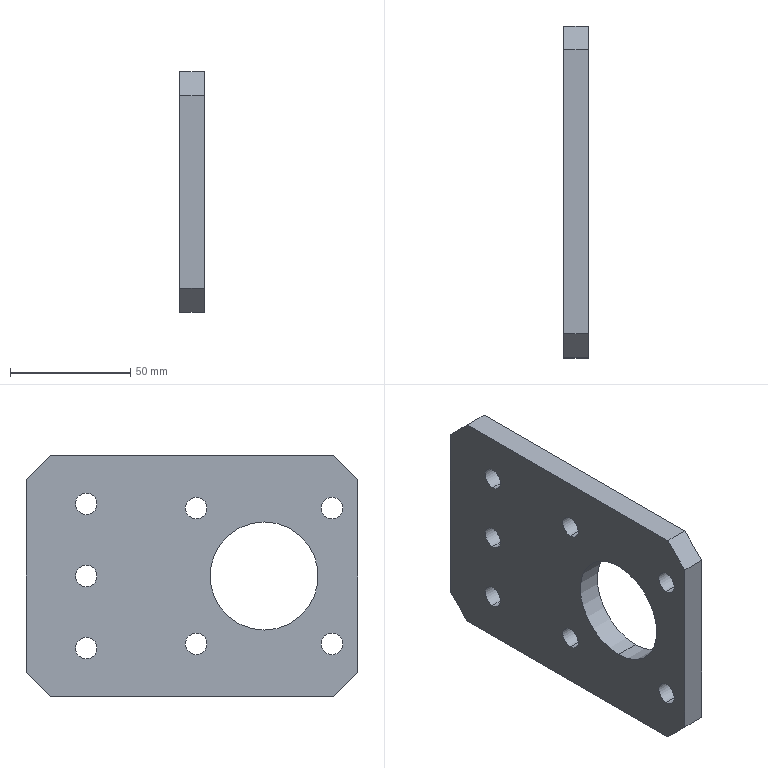Part | SolidWorks | features HoleWzd 2, Chamfer 1, CirPattern 1, Extrusion 1, ICE 1 | 1 solid | 26 faces | box 10 x 138 x 100 mm | volume 115642 mm3 | cylinder 16 | plane 10 | commonest cylinder face diameters 9 x14 45 x2
STEP:
#1=CARTESIAN_POINT('',(0.,-1.75,-23.75));
#2=VERTEX_POINT('',#1);
#3=CARTESIAN_POINT('',(0.,-1.75,-32.75));
#4=VERTEX_POINT('',#3);
#5=CARTESIAN_POINT('',(0.,-1.75,-28.25));
#6=DIRECTION('',(1.,0.,0.));
#7=DIRECTION('',(0.,0.,-1.));
#8=AXIS2_PLACEMENT_3D('',#5,#6,#7);
#9=CIRCLE('',#8,4.5);
#10=EDGE_CURVE('',#2,#4,#9,.T.);
#11=ORIENTED_EDGE('',*,*,#10,.F.);
#12=CARTESIAN_POINT('',(10.,-1.75,-23.75));
#13=VERTEX_POINT('',#12);
#14=CARTESIAN_POINT('',(10.,-1.75,-23.75));
#15=DIRECTION('',(1.,0.,0.));
#16=VECTOR('',#15,1000.);
#17=LINE('',#14,#16);
#18=EDGE_CURVE('',#2,#13,#17,.T.);
#19=ORIENTED_EDGE('',*,*,#18,.T.);
#20=CARTESIAN_POINT('',(10.,-1.75,-32.75));
#21=VERTEX_POINT('',#20);
#22=CARTESIAN_POINT('',(10.,-1.75,-28.25));
#23=DIRECTION('',(1.,0.,0.));
#24=DIRECTION('',(0.,0.,-1.));
#25=AXIS2_PLACEMENT_3D('',#22,#23,#24);
#26=CIRCLE('',#25,4.5);
#27=EDGE_CURVE('',#13,#21,#26,.T.);
#28=ORIENTED_EDGE('',*,*,#27,.T.);
#29=CARTESIAN_POINT('',(10.,-1.75,-32.75));
#30=DIRECTION('',(1.,0.,0.));
#31=VECTOR('',#30,1000.);
#32=LINE('',#29,#31);
#33=EDGE_CURVE('',#4,#21,#32,.T.);
#34=ORIENTED_EDGE('',*,*,#33,.F.);
#35=EDGE_LOOP('',(#11,#19,#28,#34));
#36=FACE_OUTER_BOUND('',#35,.T.);
#37=CARTESIAN_POINT('',(10.,-1.75,-28.25));
#38=DIRECTION('',(1.,0.,0.));
#39=DIRECTION('',(0.,0.,-1.));
#40=AXIS2_PLACEMENT_3D('',#37,#38,#39);
#41=CYLINDRICAL_SURFACE('',#40,4.5);
#42=ADVANCED_FACE('',(#36),#41,.F.);
#43=CARTESIAN_POINT('',(0.,-58.25,-23.75));
#44=VERTEX_POINT('',#43);
#45=CARTESIAN_POINT('',(0.,-58.25,-32.75));
#46=VERTEX_POINT('',#45);
#47=CARTESIAN_POINT('',(0.,-58.25,-28.25));
#48=DIRECTION('',(1.,0.,0.));
#49=DIRECTION('',(0.,0.,-1.));
#50=AXIS2_PLACEMENT_3D('',#47,#48,#49);
#51=CIRCLE('',#50,4.5);
#52=EDGE_CURVE('',#44,#46,#51,.T.);
#53=ORIENTED_EDGE('',*,*,#52,.F.);
#54=CARTESIAN_POINT('',(10.,-58.25,-23.75));
#55=VERTEX_POINT('',#54);
#56=CARTESIAN_POINT('',(10.,-58.25,-23.75));
#57=DIRECTION('',(1.,0.,0.));
#58=VECTOR('',#57,1000.);
#59=LINE('',#56,#58);
#60=EDGE_CURVE('',#44,#55,#59,.T.);
#61=ORIENTED_EDGE('',*,*,#60,.T.);
#62=CARTESIAN_POINT('',(10.,-58.25,-32.75));
#63=VERTEX_POINT('',#62);
#64=CARTESIAN_POINT('',(10.,-58.25,-28.25));
#65=DIRECTION('',(1.,0.,0.));
#66=DIRECTION('',(0.,0.,-1.));
#67=AXIS2_PLACEMENT_3D('',#64,#65,#66);
#68=CIRCLE('',#67,4.5);
#69=EDGE_CURVE('',#55,#63,#68,.T.);
#70=ORIENTED_EDGE('',*,*,#69,.T.);
#71=CARTESIAN_POINT('',(10.,-58.25,-32.75));
#72=DIRECTION('',(1.,0.,0.));
#73=VECTOR('',#72,1000.);
#74=LINE('',#71,#73);
#75=EDGE_CURVE('',#46,#63,#74,.T.);
#76=ORIENTED_EDGE('',*,*,#75,.F.);
#77=EDGE_LOOP('',(#53,#61,#70,#76));
#78=FACE_OUTER_BOUND('',#77,.T.);
#79=CARTESIAN_POINT('',(10.,-58.25,-28.25));
#80=DIRECTION('',(1.,0.,0.));
#81=DIRECTION('',(0.,0.,-1.));
#82=AXIS2_PLACEMENT_3D('',#79,#80,#81);
#83=CYLINDRICAL_SURFACE('',#82,4.5);
#84=ADVANCED_FACE('',(#78),#83,.F.);
#85=CARTESIAN_POINT('',(0.,-58.25,32.75));
#86=VERTEX_POINT('',#85);
#87=CARTESIAN_POINT('',(0.,-58.25,23.75));
#88=VERTEX_POINT('',#87);
#89=CARTESIAN_POINT('',(0.,-58.25,28.25));
#90=DIRECTION('',(1.,0.,0.));
#91=DIRECTION('',(0.,0.,-1.));
#92=AXIS2_PLACEMENT_3D('',#89,#90,#91);
#93=CIRCLE('',#92,4.5);
#94=EDGE_CURVE('',#86,#88,#93,.T.);
#95=ORIENTED_EDGE('',*,*,#94,.F.);
#96=CARTESIAN_POINT('',(10.,-58.25,32.75));
#97=VERTEX_POINT('',#96);
#98=CARTESIAN_POINT('',(10.,-58.25,32.75));
#99=DIRECTION('',(1.,0.,0.));
#100=VECTOR('',#99,1000.);
#101=LINE('',#98,#100);
#102=EDGE_CURVE('',#86,#97,#101,.T.);
#103=ORIENTED_EDGE('',*,*,#102,.T.);
#104=CARTESIAN_POINT('',(10.,-58.25,23.75));
#105=VERTEX_POINT('',#104);
#106=CARTESIAN_POINT('',(10.,-58.25,28.25));
#107=DIRECTION('',(1.,0.,0.));
#108=DIRECTION('',(0.,0.,-1.));
#109=AXIS2_PLACEMENT_3D('',#106,#107,#108);
#110=CIRCLE('',#109,4.5);
#111=EDGE_CURVE('',#97,#105,#110,.T.);
#112=ORIENTED_EDGE('',*,*,#111,.T.);
#113=CARTESIAN_POINT('',(10.,-58.25,23.75));
#114=DIRECTION('',(1.,0.,0.));
#115=VECTOR('',#114,1000.);
#116=LINE('',#113,#115);
#117=EDGE_CURVE('',#88,#105,#116,.T.);
#118=ORIENTED_EDGE('',*,*,#117,.F.);
#119=EDGE_LOOP('',(#95,#103,#112,#118));
#120=FACE_OUTER_BOUND('',#119,.T.);
#121=CARTESIAN_POINT('',(10.,-58.25,28.25));
#122=DIRECTION('',(1.,0.,0.));
#123=DIRECTION('',(0.,0.,-1.));
#124=AXIS2_PLACEMENT_3D('',#121,#122,#123);
#125=CYLINDRICAL_SURFACE('',#124,4.5);
#126=ADVANCED_FACE('',(#120),#125,.F.);
#127=CARTESIAN_POINT('',(0.,-1.75,32.75));
#128=VERTEX_POINT('',#127);
#129=CARTESIAN_POINT('',(0.,-1.75,23.75));
#130=VERTEX_POINT('',#129);
#131=CARTESIAN_POINT('',(0.,-1.75,28.25));
#132=DIRECTION('',(1.,0.,0.));
#133=DIRECTION('',(0.,0.,-1.));
#134=AXIS2_PLACEMENT_3D('',#131,#132,#133);
#135=CIRCLE('',#134,4.5);
#136=EDGE_CURVE('',#128,#130,#135,.T.);
#137=ORIENTED_EDGE('',*,*,#136,.F.);
#138=CARTESIAN_POINT('',(10.,-1.75,32.75));
#139=VERTEX_POINT('',#138);
#140=CARTESIAN_POINT('',(10.,-1.75,32.75));
#141=DIRECTION('',(1.,0.,0.));
#142=VECTOR('',#141,1000.);
#143=LINE('',#140,#142);
#144=EDGE_CURVE('',#128,#139,#143,.T.);
#145=ORIENTED_EDGE('',*,*,#144,.T.);
#146=CARTESIAN_POINT('',(10.,-1.75,23.75));
#147=VERTEX_POINT('',#146);
#148=CARTESIAN_POINT('',(10.,-1.75,28.25));
#149=DIRECTION('',(1.,0.,0.));
#150=DIRECTION('',(0.,0.,-1.));
#151=AXIS2_PLACEMENT_3D('',#148,#149,#150);
#152=CIRCLE('',#151,4.5);
#153=EDGE_CURVE('',#139,#147,#152,.T.);
#154=ORIENTED_EDGE('',*,*,#153,.T.);
#155=CARTESIAN_POINT('',(10.,-1.75,23.75));
#156=DIRECTION('',(1.,0.,0.));
#157=VECTOR('',#156,1000.);
#158=LINE('',#155,#157);
#159=EDGE_CURVE('',#130,#147,#158,.T.);
#160=ORIENTED_EDGE('',*,*,#159,.F.);
#161=EDGE_LOOP('',(#137,#145,#154,#160));
#162=FACE_OUTER_BOUND('',#161,.T.);
#163=CARTESIAN_POINT('',(10.,-1.75,28.25));
#164=DIRECTION('',(1.,0.,0.));
#165=DIRECTION('',(0.,0.,-1.));
#166=AXIS2_PLACEMENT_3D('',#163,#164,#165);
#167=CYLINDRICAL_SURFACE('',#166,4.5);
#168=ADVANCED_FACE('',(#162),#167,.F.);
#169=CARTESIAN_POINT('',(0.,-30.,22.5));
#170=VERTEX_POINT('',#169);
#171=CARTESIAN_POINT('',(0.,-30.,-22.5));
#172=VERTEX_POINT('',#171);
#173=CARTESIAN_POINT('',(0.,-30.,0.));
#174=DIRECTION('',(1.,0.,0.));
#175=DIRECTION('',(0.,0.,-1.));
#176=AXIS2_PLACEMENT_3D('',#173,#174,#175);
#177=CIRCLE('',#176,22.5);
#178=EDGE_CURVE('',#170,#172,#177,.T.);
#179=ORIENTED_EDGE('',*,*,#178,.F.);
#180=CARTESIAN_POINT('',(10.,-30.,22.5));
#181=VERTEX_POINT('',#180);
#182=CARTESIAN_POINT('',(0.,-30.,22.5));
#183=DIRECTION('',(1.,0.,0.));
#184=VECTOR('',#183,1000.);
#185=LINE('',#182,#184);
#186=EDGE_CURVE('',#170,#181,#185,.T.);
#187=ORIENTED_EDGE('',*,*,#186,.T.);
#188=CARTESIAN_POINT('',(10.,-30.,-22.5));
#189=VERTEX_POINT('',#188);
#190=CARTESIAN_POINT('',(10.,-30.,0.));
#191=DIRECTION('',(1.,0.,0.));
#192=DIRECTION('',(0.,0.,-1.));
#193=AXIS2_PLACEMENT_3D('',#190,#191,#192);
#194=CIRCLE('',#193,22.5);
#195=EDGE_CURVE('',#181,#189,#194,.T.);
#196=ORIENTED_EDGE('',*,*,#195,.T.);
#197=CARTESIAN_POINT('',(0.,-30.,-22.5));
#198=DIRECTION('',(1.,0.,0.));
#199=VECTOR('',#198,1000.);
#200=LINE('',#197,#199);
#201=EDGE_CURVE('',#172,#189,#200,.T.);
#202=ORIENTED_EDGE('',*,*,#201,.F.);
#203=EDGE_LOOP('',(#179,#187,#196,#202));
#204=FACE_OUTER_BOUND('',#203,.T.);
#205=CARTESIAN_POINT('',(0.,-30.,0.));
#206=DIRECTION('',(1.,0.,0.));
#207=DIRECTION('',(0.,0.,-1.));
#208=AXIS2_PLACEMENT_3D('',#205,#206,#207);
#209=CYLINDRICAL_SURFACE('',#208,22.5);
#210=ADVANCED_FACE('',(#204),#209,.F.);
#211=CARTESIAN_POINT('',(0.,44.,34.5));
#212=VERTEX_POINT('',#211);
#213=CARTESIAN_POINT('',(0.,44.,25.5));
#214=VERTEX_POINT('',#213);
#215=CARTESIAN_POINT('',(0.,44.,30.));
#216=DIRECTION('',(1.,0.,0.));
#217=DIRECTION('',(0.,0.,-1.));
#218=AXIS2_PLACEMENT_3D('',#215,#216,#217);
#219=CIRCLE('',#218,4.5);
#220=EDGE_CURVE('',#212,#214,#219,.T.);
#221=ORIENTED_EDGE('',*,*,#220,.F.);
#222=CARTESIAN_POINT('',(10.,44.,34.5));
#223=VERTEX_POINT('',#222);
#224=CARTESIAN_POINT('',(10.,44.,34.5));
#225=DIRECTION('',(1.,0.,0.));
#226=VECTOR('',#225,1000.);
#227=LINE('',#224,#226);
#228=EDGE_CURVE('',#212,#223,#227,.T.);
#229=ORIENTED_EDGE('',*,*,#228,.T.);
#230=CARTESIAN_POINT('',(10.,44.,25.5));
#231=VERTEX_POINT('',#230);
#232=CARTESIAN_POINT('',(10.,44.,30.));
#233=DIRECTION('',(1.,0.,0.));
#234=DIRECTION('',(0.,0.,-1.));
#235=AXIS2_PLACEMENT_3D('',#232,#233,#234);
#236=CIRCLE('',#235,4.5);
#237=EDGE_CURVE('',#223,#231,#236,.T.);
#238=ORIENTED_EDGE('',*,*,#237,.T.);
#239=CARTESIAN_POINT('',(10.,44.,25.5));
#240=DIRECTION('',(1.,0.,0.));
#241=VECTOR('',#240,1000.);
#242=LINE('',#239,#241);
#243=EDGE_CURVE('',#214,#231,#242,.T.);
#244=ORIENTED_EDGE('',*,*,#243,.F.);
#245=EDGE_LOOP('',(#221,#229,#238,#244));
#246=FACE_OUTER_BOUND('',#245,.T.);
#247=CARTESIAN_POINT('',(10.,44.,30.));
#248=DIRECTION('',(1.,0.,0.));
#249=DIRECTION('',(0.,0.,-1.));
#250=AXIS2_PLACEMENT_3D('',#247,#248,#249);
#251=CYLINDRICAL_SURFACE('',#250,4.5);
#252=ADVANCED_FACE('',(#246),#251,.F.);
#253=CARTESIAN_POINT('',(0.,44.,4.5));
#254=VERTEX_POINT('',#253);
#255=CARTESIAN_POINT('',(0.,44.,-4.5));
#256=VERTEX_POINT('',#255);
#257=CARTESIAN_POINT('',(0.,44.,0.));
#258=DIRECTION('',(1.,0.,0.));
#259=DIRECTION('',(0.,0.,-1.));
#260=AXIS2_PLACEMENT_3D('',#257,#258,#259);
#261=CIRCLE('',#260,4.5);
#262=EDGE_CURVE('',#254,#256,#261,.T.);
#263=ORIENTED_EDGE('',*,*,#262,.F.);
#264=CARTESIAN_POINT('',(10.,44.,4.5));
#265=VERTEX_POINT('',#264);
#266=CARTESIAN_POINT('',(10.,44.,4.5));
#267=DIRECTION('',(1.,0.,0.));
#268=VECTOR('',#267,1000.);
#269=LINE('',#266,#268);
#270=EDGE_CURVE('',#254,#265,#269,.T.);
#271=ORIENTED_EDGE('',*,*,#270,.T.);
#272=CARTESIAN_POINT('',(10.,44.,-4.5));
#273=VERTEX_POINT('',#272);
#274=CARTESIAN_POINT('',(10.,44.,0.));
#275=DIRECTION('',(1.,0.,0.));
#276=DIRECTION('',(0.,0.,-1.));
#277=AXIS2_PLACEMENT_3D('',#274,#275,#276);
#278=CIRCLE('',#277,4.5);
#279=EDGE_CURVE('',#265,#273,#278,.T.);
#280=ORIENTED_EDGE('',*,*,#279,.T.);
#281=CARTESIAN_POINT('',(10.,44.,-4.5));
#282=DIRECTION('',(1.,0.,0.));
#283=VECTOR('',#282,1000.);
#284=LINE('',#281,#283);
#285=EDGE_CURVE('',#256,#273,#284,.T.);
#286=ORIENTED_EDGE('',*,*,#285,.F.);
#287=EDGE_LOOP('',(#263,#271,#280,#286));
#288=FACE_OUTER_BOUND('',#287,.T.);
#289=CARTESIAN_POINT('',(10.,44.,0.));
#290=DIRECTION('',(1.,0.,0.));
#291=DIRECTION('',(0.,0.,-1.));
#292=AXIS2_PLACEMENT_3D('',#289,#290,#291);
#293=CYLINDRICAL_SURFACE('',#292,4.5);
#294=ADVANCED_FACE('',(#288),#293,.F.);
#295=CARTESIAN_POINT('',(0.,44.,-25.5));
#296=VERTEX_POINT('',#295);
#297=CARTESIAN_POINT('',(0.,44.,-34.5));
#298=VERTEX_POINT('',#297);
#299=CARTESIAN_POINT('',(0.,44.,-30.));
#300=DIRECTION('',(1.,0.,0.));
#301=DIRECTION('',(0.,0.,-1.));
#302=AXIS2_PLACEMENT_3D('',#299,#300,#301);
#303=CIRCLE('',#302,4.5);
#304=EDGE_CURVE('',#296,#298,#303,.T.);
#305=ORIENTED_EDGE('',*,*,#304,.F.);
#306=CARTESIAN_POINT('',(10.,44.,-25.5));
#307=VERTEX_POINT('',#306);
#308=CARTESIAN_POINT('',(10.,44.,-25.5));
#309=DIRECTION('',(1.,0.,0.));
#310=VECTOR('',#309,1000.);
#311=LINE('',#308,#310);
#312=EDGE_CURVE('',#296,#307,#311,.T.);
#313=ORIENTED_EDGE('',*,*,#312,.T.);
#314=CARTESIAN_POINT('',(10.,44.,-34.5));
#315=VERTEX_POINT('',#314);
#316=CARTESIAN_POINT('',(10.,44.,-30.));
#317=DIRECTION('',(1.,0.,0.));
#318=DIRECTION('',(0.,0.,-1.));
#319=AXIS2_PLACEMENT_3D('',#316,#317,#318);
#320=CIRCLE('',#319,4.5);
#321=EDGE_CURVE('',#307,#315,#320,.T.);
#322=ORIENTED_EDGE('',*,*,#321,.T.);
#323=CARTESIAN_POINT('',(10.,44.,-34.5));
#324=DIRECTION('',(1.,0.,0.));
#325=VECTOR('',#324,1000.);
#326=LINE('',#323,#325);
#327=EDGE_CURVE('',#298,#315,#326,.T.);
#328=ORIENTED_EDGE('',*,*,#327,.F.);
#329=EDGE_LOOP('',(#305,#313,#322,#328));
#330=FACE_OUTER_BOUND('',#329,.T.);
#331=CARTESIAN_POINT('',(10.,44.,-30.));
#332=DIRECTION('',(1.,0.,0.));
#333=DIRECTION('',(0.,0.,-1.));
#334=AXIS2_PLACEMENT_3D('',#331,#332,#333);
#335=CYLINDRICAL_SURFACE('',#334,4.5);
#336=ADVANCED_FACE('',(#330),#335,.F.);
#337=CARTESIAN_POINT('',(10.,-59.,-50.));
#338=VERTEX_POINT('',#337);
#339=CARTESIAN_POINT('',(10.,59.,-50.));
#340=VERTEX_POINT('',#339);
#341=CARTESIAN_POINT('',(10.,69.,-50.));
#342=DIRECTION('',(0.,1.,0.));
#343=VECTOR('',#342,1000.);
#344=LINE('',#341,#343);
#345=EDGE_CURVE('',#338,#340,#344,.T.);
#346=ORIENTED_EDGE('',*,*,#345,.F.);
#347=CARTESIAN_POINT('',(0.,-59.,-50.));
#348=VERTEX_POINT('',#347);
#349=CARTESIAN_POINT('',(10.,-59.,-50.));
#350=DIRECTION('',(-1.,0.,0.));
#351=VECTOR('',#350,1000.);
#352=LINE('',#349,#351);
#353=EDGE_CURVE('',#338,#348,#352,.T.);
#354=ORIENTED_EDGE('',*,*,#353,.T.);
#355=CARTESIAN_POINT('',(0.,59.,-50.));
#356=VERTEX_POINT('',#355);
#357=CARTESIAN_POINT('',(0.,69.,-50.));
#358=DIRECTION('',(0.,1.,0.));
#359=VECTOR('',#358,1000.);
#360=LINE('',#357,#359);
#361=EDGE_CURVE('',#348,#356,#360,.T.);
#362=ORIENTED_EDGE('',*,*,#361,.T.);
#363=CARTESIAN_POINT('',(10.,59.,-50.));
#364=DIRECTION('',(1.,0.,0.));
#365=VECTOR('',#364,1000.);
#366=LINE('',#363,#365);
#367=EDGE_CURVE('',#356,#340,#366,.T.);
#368=ORIENTED_EDGE('',*,*,#367,.T.);
#369=EDGE_LOOP('',(#346,#354,#362,#368));
#370=FACE_OUTER_BOUND('',#369,.T.);
#371=CARTESIAN_POINT('',(10.,69.,-50.));
#372=DIRECTION('',(0.,0.,1.));
#373=DIRECTION('',(0.,-1.,0.));
#374=AXIS2_PLACEMENT_3D('',#371,#372,#373);
#375=PLANE('',#374);
#376=ADVANCED_FACE('',(#370),#375,.F.);
#377=CARTESIAN_POINT('',(10.,69.,-40.));
#378=VERTEX_POINT('',#377);
#379=CARTESIAN_POINT('',(10.,69.,40.));
#380=VERTEX_POINT('',#379);
#381=CARTESIAN_POINT('',(10.,69.,50.));
#382=DIRECTION('',(0.,0.,1.));
#383=VECTOR('',#382,1000.);
#384=LINE('',#381,#383);
#385=EDGE_CURVE('',#378,#380,#384,.T.);
#386=ORIENTED_EDGE('',*,*,#385,.F.);
#387=CARTESIAN_POINT('',(0.,69.,-40.));
#388=VERTEX_POINT('',#387);
#389=CARTESIAN_POINT('',(10.,69.,-40.));
#390=DIRECTION('',(-1.,0.,0.));
#391=VECTOR('',#390,1000.);
#392=LINE('',#389,#391);
#393=EDGE_CURVE('',#378,#388,#392,.T.);
#394=ORIENTED_EDGE('',*,*,#393,.T.);
#395=CARTESIAN_POINT('',(0.,69.,40.));
#396=VERTEX_POINT('',#395);
#397=CARTESIAN_POINT('',(0.,69.,50.));
#398=DIRECTION('',(0.,0.,1.));
#399=VECTOR('',#398,1000.);
#400=LINE('',#397,#399);
#401=EDGE_CURVE('',#388,#396,#400,.T.);
#402=ORIENTED_EDGE('',*,*,#401,.T.);
#403=CARTESIAN_POINT('',(10.,69.,40.));
#404=DIRECTION('',(1.,0.,0.));
#405=VECTOR('',#404,1000.);
#406=LINE('',#403,#405);
#407=EDGE_CURVE('',#396,#380,#406,.T.);
#408=ORIENTED_EDGE('',*,*,#407,.T.);
#409=EDGE_LOOP('',(#386,#394,#402,#408));
#410=FACE_OUTER_BOUND('',#409,.T.);
#411=CARTESIAN_POINT('',(10.,69.,50.));
#412=DIRECTION('',(0.,-1.,0.));
#413=DIRECTION('',(0.,0.,-1.));
#414=AXIS2_PLACEMENT_3D('',#411,#412,#413);
#415=PLANE('',#414);
#416=ADVANCED_FACE('',(#410),#415,.F.);
#417=CARTESIAN_POINT('',(0.,59.,50.));
#418=VERTEX_POINT('',#417);
#419=CARTESIAN_POINT('',(0.,-59.,50.));
#420=VERTEX_POINT('',#419);
#421=CARTESIAN_POINT('',(0.,69.,50.));
#422=DIRECTION('',(0.,-1.,0.));
#423=VECTOR('',#422,1000.);
#424=LINE('',#421,#423);
#425=EDGE_CURVE('',#418,#420,#424,.T.);
#426=ORIENTED_EDGE('',*,*,#425,.T.);
#427=CARTESIAN_POINT('',(10.,-59.,50.));
#428=VERTEX_POINT('',#427);
#429=CARTESIAN_POINT('',(10.,-59.,50.));
#430=DIRECTION('',(1.,0.,0.));
#431=VECTOR('',#430,1000.);
#432=LINE('',#429,#431);
#433=EDGE_CURVE('',#420,#428,#432,.T.);
#434=ORIENTED_EDGE('',*,*,#433,.T.);
#435=CARTESIAN_POINT('',(10.,59.,50.));
#436=VERTEX_POINT('',#435);
#437=CARTESIAN_POINT('',(10.,69.,50.));
#438=DIRECTION('',(0.,-1.,0.));
#439=VECTOR('',#438,1000.);
#440=LINE('',#437,#439);
#441=EDGE_CURVE('',#436,#428,#440,.T.);
#442=ORIENTED_EDGE('',*,*,#441,.F.);
#443=CARTESIAN_POINT('',(10.,59.,50.));
#444=DIRECTION('',(-1.,0.,0.));
#445=VECTOR('',#444,1000.);
#446=LINE('',#443,#445);
#447=EDGE_CURVE('',#436,#418,#446,.T.);
#448=ORIENTED_EDGE('',*,*,#447,.T.);
#449=EDGE_LOOP('',(#426,#434,#442,#448));
#450=FACE_OUTER_BOUND('',#449,.T.);
#451=CARTESIAN_POINT('',(10.,69.,50.));
#452=DIRECTION('',(0.,0.,-1.));
#453=DIRECTION('',(0.,1.,0.));
#454=AXIS2_PLACEMENT_3D('',#451,#452,#453);
#455=PLANE('',#454);
#456=ADVANCED_FACE('',(#450),#455,.F.);
#457=CARTESIAN_POINT('',(10.,-69.,40.));
#458=VERTEX_POINT('',#457);
#459=CARTESIAN_POINT('',(10.,-69.,-40.));
#460=VERTEX_POINT('',#459);
#461=CARTESIAN_POINT('',(10.,-69.,50.));
#462=DIRECTION('',(0.,0.,-1.));
#463=VECTOR('',#462,1000.);
#464=LINE('',#461,#463);
#465=EDGE_CURVE('',#458,#460,#464,.T.);
#466=ORIENTED_EDGE('',*,*,#465,.F.);
#467=CARTESIAN_POINT('',(0.,-69.,40.));
#468=VERTEX_POINT('',#467);
#469=CARTESIAN_POINT('',(10.,-69.,40.));
#470=DIRECTION('',(-1.,0.,0.));
#471=VECTOR('',#470,1000.);
#472=LINE('',#469,#471);
#473=EDGE_CURVE('',#458,#468,#472,.T.);
#474=ORIENTED_EDGE('',*,*,#473,.T.);
#475=CARTESIAN_POINT('',(0.,-69.,-40.));
#476=VERTEX_POINT('',#475);
#477=CARTESIAN_POINT('',(0.,-69.,50.));
#478=DIRECTION('',(0.,0.,-1.));
#479=VECTOR('',#478,1000.);
#480=LINE('',#477,#479);
#481=EDGE_CURVE('',#468,#476,#480,.T.);
#482=ORIENTED_EDGE('',*,*,#481,.T.);
#483=CARTESIAN_POINT('',(10.,-69.,-40.));
#484=DIRECTION('',(1.,0.,0.));
#485=VECTOR('',#484,1000.);
#486=LINE('',#483,#485);
#487=EDGE_CURVE('',#476,#460,#486,.T.);
#488=ORIENTED_EDGE('',*,*,#487,.T.);
#489=EDGE_LOOP('',(#466,#474,#482,#488));
#490=FACE_OUTER_BOUND('',#489,.T.);
#491=CARTESIAN_POINT('',(10.,-69.,50.));
#492=DIRECTION('',(0.,1.,0.));
#493=DIRECTION('',(0.,0.,1.));
#494=AXIS2_PLACEMENT_3D('',#491,#492,#493);
#495=PLANE('',#494);
#496=ADVANCED_FACE('',(#490),#495,.F.);
#497=CARTESIAN_POINT('',(10.,-1.75,-28.25));
#498=DIRECTION('',(1.,0.,0.));
#499=DIRECTION('',(0.,0.,-1.));
#500=AXIS2_PLACEMENT_3D('',#497,#498,#499);
#501=CIRCLE('',#500,4.5);
#502=EDGE_CURVE('',#21,#13,#501,.T.);
#503=ORIENTED_EDGE('',*,*,#502,.F.);
#504=ORIENTED_EDGE('',*,*,#27,.F.);
#505=EDGE_LOOP('',(#503,#504));
#506=FACE_BOUND('',#505,.T.);
#507=CARTESIAN_POINT('',(10.,-58.25,-28.25));
#508=DIRECTION('',(1.,0.,0.));
#509=DIRECTION('',(0.,0.,-1.));
#510=AXIS2_PLACEMENT_3D('',#507,#508,#509);
#511=CIRCLE('',#510,4.5);
#512=EDGE_CURVE('',#63,#55,#511,.T.);
#513=ORIENTED_EDGE('',*,*,#512,.F.);
#514=ORIENTED_EDGE('',*,*,#69,.F.);
#515=EDGE_LOOP('',(#513,#514));
#516=FACE_BOUND('',#515,.T.);
#517=CARTESIAN_POINT('',(10.,-58.25,28.25));
#518=DIRECTION('',(1.,0.,0.));
#519=DIRECTION('',(0.,0.,-1.));
#520=AXIS2_PLACEMENT_3D('',#517,#518,#519);
#521=CIRCLE('',#520,4.5);
#522=EDGE_CURVE('',#105,#97,#521,.T.);
#523=ORIENTED_EDGE('',*,*,#522,.F.);
#524=ORIENTED_EDGE('',*,*,#111,.F.);
#525=EDGE_LOOP('',(#523,#524));
#526=FACE_BOUND('',#525,.T.);
#527=CARTESIAN_POINT('',(10.,-1.75,28.25));
#528=DIRECTION('',(1.,0.,0.));
#529=DIRECTION('',(0.,0.,-1.));
#530=AXIS2_PLACEMENT_3D('',#527,#528,#529);
#531=CIRCLE('',#530,4.5);
#532=EDGE_CURVE('',#147,#139,#531,.T.);
#533=ORIENTED_EDGE('',*,*,#532,.F.);
#534=ORIENTED_EDGE('',*,*,#153,.F.);
#535=EDGE_LOOP('',(#533,#534));
#536=FACE_BOUND('',#535,.T.);
#537=CARTESIAN_POINT('',(10.,-30.,0.));
#538=DIRECTION('',(1.,0.,0.));
#539=DIRECTION('',(0.,0.,-1.));
#540=AXIS2_PLACEMENT_3D('',#537,#538,#539);
#541=CIRCLE('',#540,22.5);
#542=EDGE_CURVE('',#189,#181,#541,.T.);
#543=ORIENTED_EDGE('',*,*,#542,.F.);
#544=ORIENTED_EDGE('',*,*,#195,.F.);
#545=EDGE_LOOP('',(#543,#544));
#546=FACE_BOUND('',#545,.T.);
#547=CARTESIAN_POINT('',(10.,44.,30.));
#548=DIRECTION('',(1.,0.,0.));
#549=DIRECTION('',(0.,0.,-1.));
#550=AXIS2_PLACEMENT_3D('',#547,#548,#549);
#551=CIRCLE('',#550,4.5);
#552=EDGE_CURVE('',#231,#223,#551,.T.);
#553=ORIENTED_EDGE('',*,*,#552,.F.);
#554=ORIENTED_EDGE('',*,*,#237,.F.);
#555=EDGE_LOOP('',(#553,#554));
#556=FACE_BOUND('',#555,.T.);
#557=CARTESIAN_POINT('',(10.,44.,0.));
#558=DIRECTION('',(1.,0.,0.));
#559=DIRECTION('',(0.,0.,-1.));
#560=AXIS2_PLACEMENT_3D('',#557,#558,#559);
#561=CIRCLE('',#560,4.5);
#562=EDGE_CURVE('',#273,#265,#561,.T.);
#563=ORIENTED_EDGE('',*,*,#562,.F.);
#564=ORIENTED_EDGE('',*,*,#279,.F.);
#565=EDGE_LOOP('',(#563,#564));
#566=FACE_BOUND('',#565,.T.);
#567=CARTESIAN_POINT('',(10.,44.,-30.));
#568=DIRECTION('',(1.,0.,0.));
#569=DIRECTION('',(0.,0.,-1.));
#570=AXIS2_PLACEMENT_3D('',#567,#568,#569);
#571=CIRCLE('',#570,4.5);
#572=EDGE_CURVE('',#315,#307,#571,.T.);
#573=ORIENTED_EDGE('',*,*,#572,.F.);
#574=ORIENTED_EDGE('',*,*,#321,.F.);
#575=EDGE_LOOP('',(#573,#574));
#576=FACE_BOUND('',#575,.T.);
#577=ORIENTED_EDGE('',*,*,#441,.T.);
#578=CARTESIAN_POINT('',(10.,-54.5,54.5));
#579=DIRECTION('',(0.,-0.7071,-0.7071));
#580=VECTOR('',#579,1000.);
#581=LINE('',#578,#580);
#582=EDGE_CURVE('',#428,#458,#581,.T.);
#583=ORIENTED_EDGE('',*,*,#582,.T.);
#584=ORIENTED_EDGE('',*,*,#465,.T.);
#585=CARTESIAN_POINT('',(10.,-54.5,-54.5));
#586=DIRECTION('',(0.,0.7071,-0.7071));
#587=VECTOR('',#586,1000.);
#588=LINE('',#585,#587);
#589=EDGE_CURVE('',#460,#338,#588,.T.);
#590=ORIENTED_EDGE('',*,*,#589,.T.);
#591=ORIENTED_EDGE('',*,*,#345,.T.);
#592=CARTESIAN_POINT('',(10.,54.5,-54.5));
#593=DIRECTION('',(0.,0.7071,0.7071));
#594=VECTOR('',#593,1000.);
#595=LINE('',#592,#594);
#596=EDGE_CURVE('',#340,#378,#595,.T.);
#597=ORIENTED_EDGE('',*,*,#596,.T.);
#598=ORIENTED_EDGE('',*,*,#385,.T.);
#599=CARTESIAN_POINT('',(10.,54.5,54.5));
#600=DIRECTION('',(0.,-0.7071,0.7071));
#601=VECTOR('',#600,1000.);
#602=LINE('',#599,#601);
#603=EDGE_CURVE('',#380,#436,#602,.T.);
#604=ORIENTED_EDGE('',*,*,#603,.T.);
#605=EDGE_LOOP('',(#577,#583,#584,#590,#591,#597,#598,#604));
#606=FACE_OUTER_BOUND('',#605,.T.);
#607=CARTESIAN_POINT('',(10.,0.,0.));
#608=DIRECTION('',(1.,0.,0.));
#609=DIRECTION('',(0.,0.,-1.));
#610=AXIS2_PLACEMENT_3D('',#607,#608,#609);
#611=PLANE('',#610);
#612=ADVANCED_FACE('',(#506,#516,#526,#536,#546,#556,#566,#576,#606),#611,.T.);
#613=CARTESIAN_POINT('',(0.,-1.75,-28.25));
#614=DIRECTION('',(1.,0.,0.));
#615=DIRECTION('',(0.,0.,-1.));
#616=AXIS2_PLACEMENT_3D('',#613,#614,#615);
#617=CIRCLE('',#616,4.5);
#618=EDGE_CURVE('',#4,#2,#617,.T.);
#619=ORIENTED_EDGE('',*,*,#618,.T.);
#620=ORIENTED_EDGE('',*,*,#10,.T.);
#621=EDGE_LOOP('',(#619,#620));
#622=FACE_BOUND('',#621,.T.);
#623=CARTESIAN_POINT('',(0.,-58.25,-28.25));
#624=DIRECTION('',(1.,0.,0.));
#625=DIRECTION('',(0.,0.,-1.));
#626=AXIS2_PLACEMENT_3D('',#623,#624,#625);
#627=CIRCLE('',#626,4.5);
#628=EDGE_CURVE('',#46,#44,#627,.T.);
#629=ORIENTED_EDGE('',*,*,#628,.T.);
#630=ORIENTED_EDGE('',*,*,#52,.T.);
#631=EDGE_LOOP('',(#629,#630));
#632=FACE_BOUND('',#631,.T.);
#633=CARTESIAN_POINT('',(0.,-58.25,28.25));
#634=DIRECTION('',(1.,0.,0.));
#635=DIRECTION('',(0.,0.,-1.));
#636=AXIS2_PLACEMENT_3D('',#633,#634,#635);
#637=CIRCLE('',#636,4.5);
#638=EDGE_CURVE('',#88,#86,#637,.T.);
#639=ORIENTED_EDGE('',*,*,#638,.T.);
#640=ORIENTED_EDGE('',*,*,#94,.T.);
#641=EDGE_LOOP('',(#639,#640));
#642=FACE_BOUND('',#641,.T.);
#643=CARTESIAN_POINT('',(0.,-1.75,28.25));
#644=DIRECTION('',(1.,0.,0.));
#645=DIRECTION('',(0.,0.,-1.));
#646=AXIS2_PLACEMENT_3D('',#643,#644,#645);
#647=CIRCLE('',#646,4.5);
#648=EDGE_CURVE('',#130,#128,#647,.T.);
#649=ORIENTED_EDGE('',*,*,#648,.T.);
#650=ORIENTED_EDGE('',*,*,#136,.T.);
#651=EDGE_LOOP('',(#649,#650));
#652=FACE_BOUND('',#651,.T.);
#653=CARTESIAN_POINT('',(0.,-30.,0.));
#654=DIRECTION('',(1.,0.,0.));
#655=DIRECTION('',(0.,0.,-1.));
#656=AXIS2_PLACEMENT_3D('',#653,#654,#655);
#657=CIRCLE('',#656,22.5);
#658=EDGE_CURVE('',#172,#170,#657,.T.);
#659=ORIENTED_EDGE('',*,*,#658,.T.);
#660=ORIENTED_EDGE('',*,*,#178,.T.);
#661=EDGE_LOOP('',(#659,#660));
#662=FACE_BOUND('',#661,.T.);
#663=CARTESIAN_POINT('',(0.,44.,30.));
#664=DIRECTION('',(1.,0.,0.));
#665=DIRECTION('',(0.,0.,-1.));
#666=AXIS2_PLACEMENT_3D('',#663,#664,#665);
#667=CIRCLE('',#666,4.5);
#668=EDGE_CURVE('',#214,#212,#667,.T.);
#669=ORIENTED_EDGE('',*,*,#668,.T.);
#670=ORIENTED_EDGE('',*,*,#220,.T.);
#671=EDGE_LOOP('',(#669,#670));
#672=FACE_BOUND('',#671,.T.);
#673=CARTESIAN_POINT('',(0.,44.,0.));
#674=DIRECTION('',(1.,0.,0.));
#675=DIRECTION('',(0.,0.,-1.));
#676=AXIS2_PLACEMENT_3D('',#673,#674,#675);
#677=CIRCLE('',#676,4.5);
#678=EDGE_CURVE('',#256,#254,#677,.T.);
#679=ORIENTED_EDGE('',*,*,#678,.T.);
#680=ORIENTED_EDGE('',*,*,#262,.T.);
#681=EDGE_LOOP('',(#679,#680));
#682=FACE_BOUND('',#681,.T.);
#683=CARTESIAN_POINT('',(0.,44.,-30.));
#684=DIRECTION('',(1.,0.,0.));
#685=DIRECTION('',(0.,0.,-1.));
#686=AXIS2_PLACEMENT_3D('',#683,#684,#685);
#687=CIRCLE('',#686,4.5);
#688=EDGE_CURVE('',#298,#296,#687,.T.);
#689=ORIENTED_EDGE('',*,*,#688,.T.);
#690=ORIENTED_EDGE('',*,*,#304,.T.);
#691=EDGE_LOOP('',(#689,#690));
#692=FACE_BOUND('',#691,.T.);
#693=ORIENTED_EDGE('',*,*,#481,.F.);
#694=CARTESIAN_POINT('',(0.,-69.,40.));
#695=DIRECTION('',(0.,0.7071,0.7071));
#696=VECTOR('',#695,1000.);
#697=LINE('',#694,#696);
#698=EDGE_CURVE('',#468,#420,#697,.T.);
#699=ORIENTED_EDGE('',*,*,#698,.T.);
#700=ORIENTED_EDGE('',*,*,#425,.F.);
#701=CARTESIAN_POINT('',(0.,59.,50.));
#702=DIRECTION('',(0.,0.7071,-0.7071));
#703=VECTOR('',#702,1000.);
#704=LINE('',#701,#703);
#705=EDGE_CURVE('',#418,#396,#704,.T.);
#706=ORIENTED_EDGE('',*,*,#705,.T.);
#707=ORIENTED_EDGE('',*,*,#401,.F.);
#708=CARTESIAN_POINT('',(0.,69.,-40.));
#709=DIRECTION('',(0.,-0.7071,-0.7071));
#710=VECTOR('',#709,1000.);
#711=LINE('',#708,#710);
#712=EDGE_CURVE('',#388,#356,#711,.T.);
#713=ORIENTED_EDGE('',*,*,#712,.T.);
#714=ORIENTED_EDGE('',*,*,#361,.F.);
#715=CARTESIAN_POINT('',(0.,-59.,-50.));
#716=DIRECTION('',(0.,-0.7071,0.7071));
#717=VECTOR('',#716,1000.);
#718=LINE('',#715,#717);
#719=EDGE_CURVE('',#348,#476,#718,.T.);
#720=ORIENTED_EDGE('',*,*,#719,.T.);
#721=EDGE_LOOP('',(#693,#699,#700,#706,#707,#713,#714,#720));
#722=FACE_OUTER_BOUND('',#721,.T.);
#723=CARTESIAN_POINT('',(0.,0.,0.));
#724=DIRECTION('',(1.,0.,0.));
#725=DIRECTION('',(0.,0.,-1.));
#726=AXIS2_PLACEMENT_3D('',#723,#724,#725);
#727=PLANE('',#726);
#728=ADVANCED_FACE('',(#622,#632,#642,#652,#662,#672,#682,#692,#722),#727,.F.);
#729=ORIENTED_EDGE('',*,*,#312,.F.);
#730=ORIENTED_EDGE('',*,*,#688,.F.);
#731=ORIENTED_EDGE('',*,*,#327,.T.);
#732=ORIENTED_EDGE('',*,*,#572,.T.);
#733=EDGE_LOOP('',(#729,#730,#731,#732));
#734=FACE_OUTER_BOUND('',#733,.T.);
#735=CARTESIAN_POINT('',(10.,44.,-30.));
#736=DIRECTION('',(1.,0.,0.));
#737=DIRECTION('',(0.,0.,-1.));
#738=AXIS2_PLACEMENT_3D('',#735,#736,#737);
#739=CYLINDRICAL_SURFACE('',#738,4.5);
#740=ADVANCED_FACE('',(#734),#739,.F.);
#741=ORIENTED_EDGE('',*,*,#270,.F.);
#742=ORIENTED_EDGE('',*,*,#678,.F.);
#743=ORIENTED_EDGE('',*,*,#285,.T.);
#744=ORIENTED_EDGE('',*,*,#562,.T.);
#745=EDGE_LOOP('',(#741,#742,#743,#744));
#746=FACE_OUTER_BOUND('',#745,.T.);
#747=CARTESIAN_POINT('',(10.,44.,0.));
#748=DIRECTION('',(1.,0.,0.));
#749=DIRECTION('',(0.,0.,-1.));
#750=AXIS2_PLACEMENT_3D('',#747,#748,#749);
#751=CYLINDRICAL_SURFACE('',#750,4.5);
#752=ADVANCED_FACE('',(#746),#751,.F.);
#753=ORIENTED_EDGE('',*,*,#228,.F.);
#754=ORIENTED_EDGE('',*,*,#668,.F.);
#755=ORIENTED_EDGE('',*,*,#243,.T.);
#756=ORIENTED_EDGE('',*,*,#552,.T.);
#757=EDGE_LOOP('',(#753,#754,#755,#756));
#758=FACE_OUTER_BOUND('',#757,.T.);
#759=CARTESIAN_POINT('',(10.,44.,30.));
#760=DIRECTION('',(1.,0.,0.));
#761=DIRECTION('',(0.,0.,-1.));
#762=AXIS2_PLACEMENT_3D('',#759,#760,#761);
#763=CYLINDRICAL_SURFACE('',#762,4.5);
#764=ADVANCED_FACE('',(#758),#763,.F.);
#765=ORIENTED_EDGE('',*,*,#186,.F.);
#766=ORIENTED_EDGE('',*,*,#658,.F.);
#767=ORIENTED_EDGE('',*,*,#201,.T.);
#768=ORIENTED_EDGE('',*,*,#542,.T.);
#769=EDGE_LOOP('',(#765,#766,#767,#768));
#770=FACE_OUTER_BOUND('',#769,.T.);
#771=CARTESIAN_POINT('',(0.,-30.,0.));
#772=DIRECTION('',(1.,0.,0.));
#773=DIRECTION('',(0.,0.,-1.));
#774=AXIS2_PLACEMENT_3D('',#771,#772,#773);
#775=CYLINDRICAL_SURFACE('',#774,22.5);
#776=ADVANCED_FACE('',(#770),#775,.F.);
#777=ORIENTED_EDGE('',*,*,#144,.F.);
#778=ORIENTED_EDGE('',*,*,#648,.F.);
#779=ORIENTED_EDGE('',*,*,#159,.T.);
#780=ORIENTED_EDGE('',*,*,#532,.T.);
#781=EDGE_LOOP('',(#777,#778,#779,#780));
#782=FACE_OUTER_BOUND('',#781,.T.);
#783=CARTESIAN_POINT('',(10.,-1.75,28.25));
#784=DIRECTION('',(1.,0.,0.));
#785=DIRECTION('',(0.,0.,-1.));
#786=AXIS2_PLACEMENT_3D('',#783,#784,#785);
#787=CYLINDRICAL_SURFACE('',#786,4.5);
#788=ADVANCED_FACE('',(#782),#787,.F.);
#789=ORIENTED_EDGE('',*,*,#102,.F.);
#790=ORIENTED_EDGE('',*,*,#638,.F.);
#791=ORIENTED_EDGE('',*,*,#117,.T.);
#792=ORIENTED_EDGE('',*,*,#522,.T.);
#793=EDGE_LOOP('',(#789,#790,#791,#792));
#794=FACE_OUTER_BOUND('',#793,.T.);
#795=CARTESIAN_POINT('',(10.,-58.25,28.25));
#796=DIRECTION('',(1.,0.,0.));
#797=DIRECTION('',(0.,0.,-1.));
#798=AXIS2_PLACEMENT_3D('',#795,#796,#797);
#799=CYLINDRICAL_SURFACE('',#798,4.5);
#800=ADVANCED_FACE('',(#794),#799,.F.);
#801=ORIENTED_EDGE('',*,*,#60,.F.);
#802=ORIENTED_EDGE('',*,*,#628,.F.);
#803=ORIENTED_EDGE('',*,*,#75,.T.);
#804=ORIENTED_EDGE('',*,*,#512,.T.);
#805=EDGE_LOOP('',(#801,#802,#803,#804));
#806=FACE_OUTER_BOUND('',#805,.T.);
#807=CARTESIAN_POINT('',(10.,-58.25,-28.25));
#808=DIRECTION('',(1.,0.,0.));
#809=DIRECTION('',(0.,0.,-1.));
#810=AXIS2_PLACEMENT_3D('',#807,#808,#809);
#811=CYLINDRICAL_SURFACE('',#810,4.5);
#812=ADVANCED_FACE('',(#806),#811,.F.);
#813=ORIENTED_EDGE('',*,*,#18,.F.);
#814=ORIENTED_EDGE('',*,*,#618,.F.);
#815=ORIENTED_EDGE('',*,*,#33,.T.);
#816=ORIENTED_EDGE('',*,*,#502,.T.);
#817=EDGE_LOOP('',(#813,#814,#815,#816));
#818=FACE_OUTER_BOUND('',#817,.T.);
#819=CARTESIAN_POINT('',(10.,-1.75,-28.25));
#820=DIRECTION('',(1.,0.,0.));
#821=DIRECTION('',(0.,0.,-1.));
#822=AXIS2_PLACEMENT_3D('',#819,#820,#821);
#823=CYLINDRICAL_SURFACE('',#822,4.5);
#824=ADVANCED_FACE('',(#818),#823,.F.);
#825=ORIENTED_EDGE('',*,*,#582,.F.);
#826=ORIENTED_EDGE('',*,*,#433,.F.);
#827=ORIENTED_EDGE('',*,*,#698,.F.);
#828=ORIENTED_EDGE('',*,*,#473,.F.);
#829=EDGE_LOOP('',(#825,#826,#827,#828));
#830=FACE_OUTER_BOUND('',#829,.T.);
#831=CARTESIAN_POINT('',(10.,-69.,40.));
#832=DIRECTION('',(0.,0.7071,-0.7071));
#833=DIRECTION('',(-1.,0.,0.));
#834=AXIS2_PLACEMENT_3D('',#831,#832,#833);
#835=PLANE('',#834);
#836=ADVANCED_FACE('',(#830),#835,.F.);
#837=ORIENTED_EDGE('',*,*,#589,.F.);
#838=ORIENTED_EDGE('',*,*,#487,.F.);
#839=ORIENTED_EDGE('',*,*,#719,.F.);
#840=ORIENTED_EDGE('',*,*,#353,.F.);
#841=EDGE_LOOP('',(#837,#838,#839,#840));
#842=FACE_OUTER_BOUND('',#841,.T.);
#843=CARTESIAN_POINT('',(10.,-59.,-50.));
#844=DIRECTION('',(0.,0.7071,0.7071));
#845=DIRECTION('',(-1.,0.,0.));
#846=AXIS2_PLACEMENT_3D('',#843,#844,#845);
#847=PLANE('',#846);
#848=ADVANCED_FACE('',(#842),#847,.F.);
#849=ORIENTED_EDGE('',*,*,#596,.F.);
#850=ORIENTED_EDGE('',*,*,#367,.F.);
#851=ORIENTED_EDGE('',*,*,#712,.F.);
#852=ORIENTED_EDGE('',*,*,#393,.F.);
#853=EDGE_LOOP('',(#849,#850,#851,#852));
#854=FACE_OUTER_BOUND('',#853,.T.);
#855=CARTESIAN_POINT('',(10.,69.,-40.));
#856=DIRECTION('',(0.,-0.7071,0.7071));
#857=DIRECTION('',(-1.,0.,0.));
#858=AXIS2_PLACEMENT_3D('',#855,#856,#857);
#859=PLANE('',#858);
#860=ADVANCED_FACE('',(#854),#859,.F.);
#861=ORIENTED_EDGE('',*,*,#603,.F.);
#862=ORIENTED_EDGE('',*,*,#407,.F.);
#863=ORIENTED_EDGE('',*,*,#705,.F.);
#864=ORIENTED_EDGE('',*,*,#447,.F.);
#865=EDGE_LOOP('',(#861,#862,#863,#864));
#866=FACE_OUTER_BOUND('',#865,.T.);
#867=CARTESIAN_POINT('',(10.,59.,50.));
#868=DIRECTION('',(0.,-0.7071,-0.7071));
#869=DIRECTION('',(-1.,0.,0.));
#870=AXIS2_PLACEMENT_3D('',#867,#868,#869);
#871=PLANE('',#870);
#872=ADVANCED_FACE('',(#866),#871,.F.);
#873=CLOSED_SHELL('',(#42,#84,#126,#168,#210,#252,#294,#336,#376,#416,#456,#496,#612,#728,#740,#752,#764,#776,#788,#800,#812,#824,#836,#848,#860,#872));
#874=MANIFOLD_SOLID_BREP('',#873);
#875=CARTESIAN_POINT('',(0.,0.,0.));
#876=DIRECTION('',(0.,0.,1.));
#877=DIRECTION('',(1.,0.,0.));
#878=AXIS2_PLACEMENT_3D('',#875,#876,#877);
#879=(LENGTH_UNIT()NAMED_UNIT(*)SI_UNIT(.MILLI.,.METRE.));
#880=UNCERTAINTY_MEASURE_WITH_UNIT(LENGTH_MEASURE(0.00001),#879,'','');
#881=(NAMED_UNIT(*)PLANE_ANGLE_UNIT()SI_UNIT($,.RADIAN.));
#882=(NAMED_UNIT(*)SI_UNIT($,.STERADIAN.)SOLID_ANGLE_UNIT());
#883=(GEOMETRIC_REPRESENTATION_CONTEXT(3)GLOBAL_UNCERTAINTY_ASSIGNED_CONTEXT((#880))GLOBAL_UNIT_ASSIGNED_CONTEXT((#879,#881,#882))REPRESENTATION_CONTEXT('',''));
#884=ADVANCED_BREP_SHAPE_REPRESENTATION('',(#874,#878),#883);